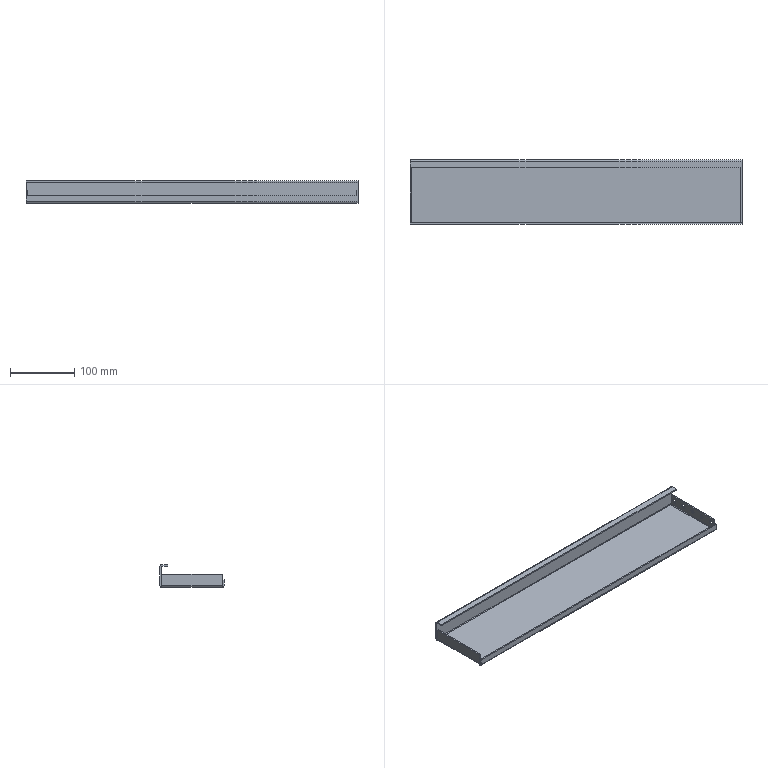Part | SolidWorks | features EdgeFlange 4, FlatPattern 1, ICE 1, SMBaseFlange 1, SheetMetal 1 | 1 solid | 60 faces | box 517 x 100 x 35 mm | volume 161621 mm3 | plane 40 | cylinder 20 | commonest cylinder face diameters 6.8 x10 2 x5 6 x5